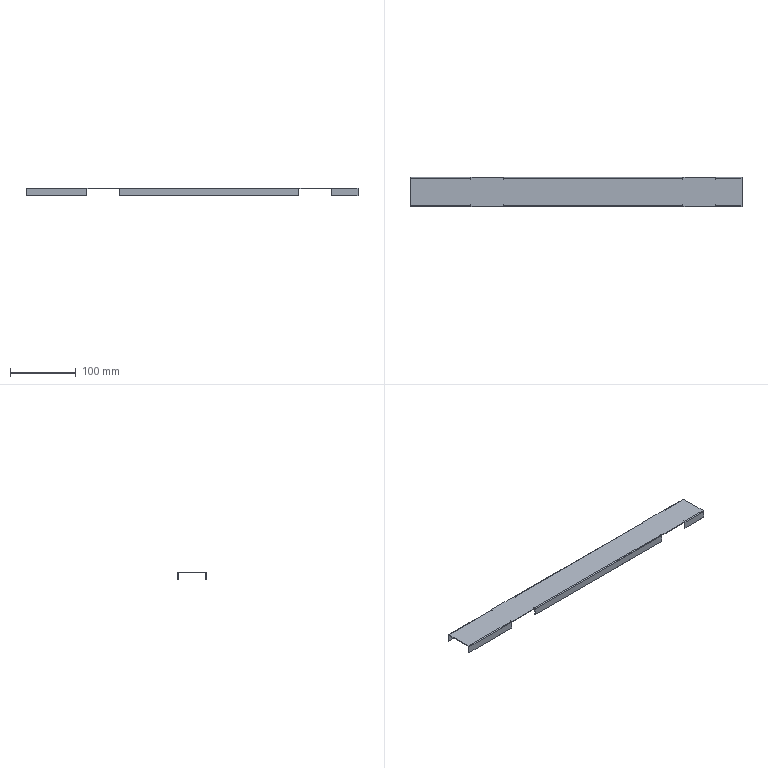Part | 1 solid | 86 faces | box 503.5 x 44 x 12 mm | volume 30777 mm3 | plane 74 | cylinder 12 | commonest cylinder face diameters 0.4 x6 2.4 x6